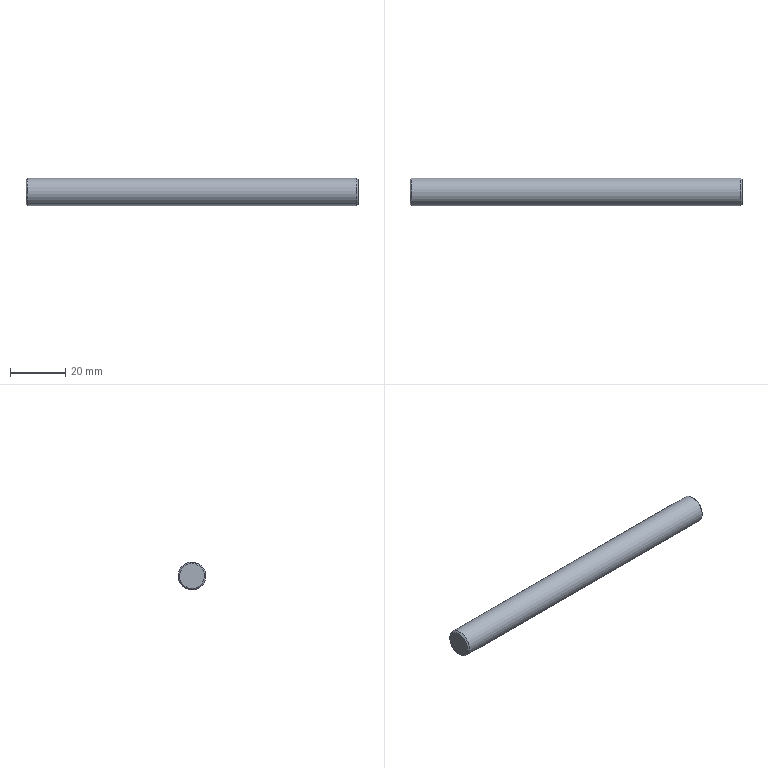Part | STEP file | SN10_016_003_EIXO | 1 solid | 5 faces | box 120 x 10 x 10 mm | volume 9417 mm3 | plane 2 | cone 2 | cylinder 1 | commonest cylinder face diameters 10 x1
STEP:
#1=CARTESIAN_POINT('',(0.,0.,0.));
#2=DIRECTION('',(0.,0.,1.));
#3=DIRECTION('',(1.,0.,0.));
#4=AXIS2_PLACEMENT_3D('',#1,#2,#3);
#5=CARTESIAN_POINT('',(5444.,-1247.157,76.449));
#6=VERTEX_POINT('',#5);
#7=CARTESIAN_POINT('',(5444.,-1245.,72.5));
#8=DIRECTION('',(1.,0.,0.));
#9=DIRECTION('',(0.,1.,0.));
#10=AXIS2_PLACEMENT_3D('',#7,#8,#9);
#11=CIRCLE('',#10,4.5);
#12=CARTESIAN_POINT('',(5444.,-1245.,72.5));
#13=DIRECTION('',(1.,0.,0.));
#14=DIRECTION('',(0.,0.,-1.));
#15=AXIS2_PLACEMENT_3D('',#12,#13,#14);
#16=PLANE('',#15);
#17=CARTESIAN_POINT('',(0.,0.));
#18=DIRECTION('',(0.,1.));
#19=AXIS2_PLACEMENT_2D('',#17,#18);
#20=CIRCLE('',#19,4.5);
#21=(GEOMETRIC_REPRESENTATION_CONTEXT(2)PARAMETRIC_REPRESENTATION_CONTEXT()REPRESENTATION_CONTEXT('',''));
#22=DEFINITIONAL_REPRESENTATION('',(#20),#21);
#23=PCURVE('',#16,#22);
#24=CARTESIAN_POINT('',(5447.5,-1245.,72.5));
#25=DIRECTION('',(-1.,0.,0.));
#26=DIRECTION('',(0.,0.1094,-0.994));
#27=AXIS2_PLACEMENT_3D('',#24,#25,#26);
#28=CONICAL_SURFACE('',#27,1.,0.7854);
#29=CARTESIAN_POINT('',(11.105,3.5));
#30=DIRECTION('',(-1.,0.));
#31=VECTOR('',#30,1.);
#32=LINE('',#29,#31);
#33=(GEOMETRIC_REPRESENTATION_CONTEXT(2)PARAMETRIC_REPRESENTATION_CONTEXT()REPRESENTATION_CONTEXT('',''));
#34=DEFINITIONAL_REPRESENTATION('',(#32),#33);
#35=PCURVE('',#28,#34);
#36=SURFACE_CURVE('',#11,(#23,#35),.PCURVE_S1.);
#37=EDGE_CURVE('',#6,#6,#36,.T.);
#38=ORIENTED_EDGE('',*,*,#37,.T.);
#39=EDGE_LOOP('',(#38));
#40=FACE_BOUND('',#39,.T.);
#41=ADVANCED_FACE('',(#40),#16,.T.);
#42=ORIENTED_EDGE('',*,*,#37,.F.);
#43=CARTESIAN_POINT('',(5443.5,-1247.397,76.888));
#44=VERTEX_POINT('',#43);
#45=CARTESIAN_POINT('',(5444.,-1247.157,76.449));
#46=CARTESIAN_POINT('',(5443.5,-1247.397,76.888));
#47=B_SPLINE_CURVE_WITH_KNOTS('',1,(#45,#46),.UNSPECIFIED.,.F.,.F.,(2,2),(4.95,5.657),.PIECEWISE_BEZIER_KNOTS.);
#48=CARTESIAN_POINT('',(9.034,0.));
#49=DIRECTION('',(0.,1.));
#50=VECTOR('',#49,1.);
#51=LINE('',#48,#50);
#52=(GEOMETRIC_REPRESENTATION_CONTEXT(2)PARAMETRIC_REPRESENTATION_CONTEXT()REPRESENTATION_CONTEXT('',''));
#53=DEFINITIONAL_REPRESENTATION('',(#51),#52);
#54=PCURVE('',#28,#53);
#55=CARTESIAN_POINT('',(2.751,0.));
#56=DIRECTION('',(0.,1.));
#57=VECTOR('',#56,1.);
#58=LINE('',#55,#57);
#59=(GEOMETRIC_REPRESENTATION_CONTEXT(2)PARAMETRIC_REPRESENTATION_CONTEXT()REPRESENTATION_CONTEXT('',''));
#60=DEFINITIONAL_REPRESENTATION('',(#58),#59);
#61=PCURVE('',#28,#60);
#62=SEAM_CURVE('',#47,(#54,#61),.PCURVE_S1.);
#63=EDGE_CURVE('',#6,#44,#62,.T.);
#64=ORIENTED_EDGE('',*,*,#63,.T.);
#65=CARTESIAN_POINT('',(5443.5,-1245.,72.5));
#66=DIRECTION('',(1.,0.,0.));
#67=DIRECTION('',(0.,1.,0.));
#68=AXIS2_PLACEMENT_3D('',#65,#66,#67);
#69=CIRCLE('',#68,5.);
#70=CARTESIAN_POINT('',(11.105,4.));
#71=DIRECTION('',(-1.,0.));
#72=VECTOR('',#71,1.);
#73=LINE('',#70,#72);
#74=(GEOMETRIC_REPRESENTATION_CONTEXT(2)PARAMETRIC_REPRESENTATION_CONTEXT()REPRESENTATION_CONTEXT('',''));
#75=DEFINITIONAL_REPRESENTATION('',(#73),#74);
#76=PCURVE('',#28,#75);
#77=CARTESIAN_POINT('',(5384.,-1245.,72.5));
#78=DIRECTION('',(1.,0.,0.));
#79=DIRECTION('',(0.,-0.4794,0.8776));
#80=AXIS2_PLACEMENT_3D('',#77,#78,#79);
#81=CYLINDRICAL_SURFACE('',#80,5.);
#82=CARTESIAN_POINT('',(-2.071,59.5));
#83=DIRECTION('',(1.,0.));
#84=VECTOR('',#83,1.);
#85=LINE('',#82,#84);
#86=(GEOMETRIC_REPRESENTATION_CONTEXT(2)PARAMETRIC_REPRESENTATION_CONTEXT()REPRESENTATION_CONTEXT('',''));
#87=DEFINITIONAL_REPRESENTATION('',(#85),#86);
#88=PCURVE('',#81,#87);
#89=SURFACE_CURVE('',#69,(#76,#88),.PCURVE_S1.);
#90=EDGE_CURVE('',#44,#44,#89,.T.);
#91=ORIENTED_EDGE('',*,*,#90,.T.);
#92=ORIENTED_EDGE('',*,*,#63,.F.);
#93=EDGE_LOOP('',(#42,#64,#91,#92));
#94=FACE_BOUND('',#93,.T.);
#95=ADVANCED_FACE('',(#94),#28,.T.);
#96=CARTESIAN_POINT('',(5324.,-1247.157,76.449));
#97=VERTEX_POINT('',#96);
#98=CARTESIAN_POINT('',(5324.,-1245.,72.5));
#99=DIRECTION('',(1.,0.,0.));
#100=DIRECTION('',(0.,1.,0.));
#101=AXIS2_PLACEMENT_3D('',#98,#99,#100);
#102=CIRCLE('',#101,4.5);
#103=CARTESIAN_POINT('',(5324.,-1245.,77.5));
#104=DIRECTION('',(1.,0.,0.));
#105=DIRECTION('',(0.,0.,-1.));
#106=AXIS2_PLACEMENT_3D('',#103,#104,#105);
#107=PLANE('',#106);
#108=CARTESIAN_POINT('',(5.,0.));
#109=DIRECTION('',(0.,1.));
#110=AXIS2_PLACEMENT_2D('',#108,#109);
#111=CIRCLE('',#110,4.5);
#112=(GEOMETRIC_REPRESENTATION_CONTEXT(2)PARAMETRIC_REPRESENTATION_CONTEXT()REPRESENTATION_CONTEXT('',''));
#113=DEFINITIONAL_REPRESENTATION('',(#111),#112);
#114=PCURVE('',#107,#113);
#115=CARTESIAN_POINT('',(5320.5,-1245.,72.5));
#116=DIRECTION('',(1.,0.,0.));
#117=DIRECTION('',(0.,-0.128,-0.9918));
#118=AXIS2_PLACEMENT_3D('',#115,#116,#117);
#119=CONICAL_SURFACE('',#118,1.,0.7854);
#120=CARTESIAN_POINT('',(1.699,3.5));
#121=DIRECTION('',(1.,0.));
#122=VECTOR('',#121,1.);
#123=LINE('',#120,#122);
#124=(GEOMETRIC_REPRESENTATION_CONTEXT(2)PARAMETRIC_REPRESENTATION_CONTEXT()REPRESENTATION_CONTEXT('',''));
#125=DEFINITIONAL_REPRESENTATION('',(#123),#124);
#126=PCURVE('',#119,#125);
#127=SURFACE_CURVE('',#102,(#114,#126),.PCURVE_S1.);
#128=EDGE_CURVE('',#97,#97,#127,.T.);
#129=ORIENTED_EDGE('',*,*,#128,.F.);
#130=EDGE_LOOP('',(#129));
#131=FACE_BOUND('',#130,.T.);
#132=ADVANCED_FACE('',(#131),#107,.F.);
#133=CARTESIAN_POINT('',(5324.5,-1247.397,76.888));
#134=VERTEX_POINT('',#133);
#135=CARTESIAN_POINT('',(5324.5,-1245.,72.5));
#136=DIRECTION('',(1.,0.,0.));
#137=DIRECTION('',(0.,1.,0.));
#138=AXIS2_PLACEMENT_3D('',#135,#136,#137);
#139=CIRCLE('',#138,5.);
#140=CARTESIAN_POINT('',(-2.071,-59.5));
#141=DIRECTION('',(1.,0.));
#142=VECTOR('',#141,1.);
#143=LINE('',#140,#142);
#144=(GEOMETRIC_REPRESENTATION_CONTEXT(2)PARAMETRIC_REPRESENTATION_CONTEXT()REPRESENTATION_CONTEXT('',''));
#145=DEFINITIONAL_REPRESENTATION('',(#143),#144);
#146=PCURVE('',#81,#145);
#147=CARTESIAN_POINT('',(1.699,4.));
#148=DIRECTION('',(1.,0.));
#149=VECTOR('',#148,1.);
#150=LINE('',#147,#149);
#151=(GEOMETRIC_REPRESENTATION_CONTEXT(2)PARAMETRIC_REPRESENTATION_CONTEXT()REPRESENTATION_CONTEXT('',''));
#152=DEFINITIONAL_REPRESENTATION('',(#150),#151);
#153=PCURVE('',#119,#152);
#154=SURFACE_CURVE('',#139,(#146,#153),.PCURVE_S1.);
#155=EDGE_CURVE('',#134,#134,#154,.T.);
#156=ORIENTED_EDGE('',*,*,#155,.T.);
#157=CARTESIAN_POINT('',(5324.5,-1247.397,76.888));
#158=CARTESIAN_POINT('',(5443.5,-1247.397,76.888));
#159=B_SPLINE_CURVE_WITH_KNOTS('',1,(#157,#158),.UNSPECIFIED.,.F.,.F.,(2,2),(-59.5,59.5),.PIECEWISE_BEZIER_KNOTS.);
#160=CARTESIAN_POINT('',(6.283,0.));
#161=DIRECTION('',(0.,1.));
#162=VECTOR('',#161,1.);
#163=LINE('',#160,#162);
#164=(GEOMETRIC_REPRESENTATION_CONTEXT(2)PARAMETRIC_REPRESENTATION_CONTEXT()REPRESENTATION_CONTEXT('',''));
#165=DEFINITIONAL_REPRESENTATION('',(#163),#164);
#166=PCURVE('',#81,#165);
#167=CARTESIAN_POINT('',(0.,0.));
#168=DIRECTION('',(0.,1.));
#169=VECTOR('',#168,1.);
#170=LINE('',#167,#169);
#171=(GEOMETRIC_REPRESENTATION_CONTEXT(2)PARAMETRIC_REPRESENTATION_CONTEXT()REPRESENTATION_CONTEXT('',''));
#172=DEFINITIONAL_REPRESENTATION('',(#170),#171);
#173=PCURVE('',#81,#172);
#174=SEAM_CURVE('',#159,(#166,#173),.PCURVE_S1.);
#175=EDGE_CURVE('',#134,#44,#174,.T.);
#176=ORIENTED_EDGE('',*,*,#175,.T.);
#177=ORIENTED_EDGE('',*,*,#90,.F.);
#178=ORIENTED_EDGE('',*,*,#175,.F.);
#179=EDGE_LOOP('',(#156,#176,#177,#178));
#180=FACE_BOUND('',#179,.T.);
#181=ADVANCED_FACE('',(#180),#81,.T.);
#182=ORIENTED_EDGE('',*,*,#155,.F.);
#183=CARTESIAN_POINT('',(5324.,-1247.157,76.449));
#184=CARTESIAN_POINT('',(5324.5,-1247.397,76.888));
#185=B_SPLINE_CURVE_WITH_KNOTS('',1,(#183,#184),.UNSPECIFIED.,.F.,.F.,(2,2),(4.95,5.657),.PIECEWISE_BEZIER_KNOTS.);
#186=CARTESIAN_POINT('',(3.77,0.));
#187=DIRECTION('',(0.,1.));
#188=VECTOR('',#187,1.);
#189=LINE('',#186,#188);
#190=(GEOMETRIC_REPRESENTATION_CONTEXT(2)PARAMETRIC_REPRESENTATION_CONTEXT()REPRESENTATION_CONTEXT('',''));
#191=DEFINITIONAL_REPRESENTATION('',(#189),#190);
#192=PCURVE('',#119,#191);
#193=CARTESIAN_POINT('',(10.053,0.));
#194=DIRECTION('',(0.,1.));
#195=VECTOR('',#194,1.);
#196=LINE('',#193,#195);
#197=(GEOMETRIC_REPRESENTATION_CONTEXT(2)PARAMETRIC_REPRESENTATION_CONTEXT()REPRESENTATION_CONTEXT('',''));
#198=DEFINITIONAL_REPRESENTATION('',(#196),#197);
#199=PCURVE('',#119,#198);
#200=SEAM_CURVE('',#185,(#192,#199),.PCURVE_S1.);
#201=EDGE_CURVE('',#97,#134,#200,.T.);
#202=ORIENTED_EDGE('',*,*,#201,.F.);
#203=ORIENTED_EDGE('',*,*,#128,.T.);
#204=ORIENTED_EDGE('',*,*,#201,.T.);
#205=EDGE_LOOP('',(#182,#202,#203,#204));
#206=FACE_BOUND('',#205,.T.);
#207=ADVANCED_FACE('',(#206),#119,.T.);
#208=CLOSED_SHELL('',(#41,#95,#132,#181,#207));
#209=MANIFOLD_SOLID_BREP('',#208);
#210=(LENGTH_UNIT()NAMED_UNIT(*)SI_UNIT(.MILLI.,.METRE.));
#211=UNCERTAINTY_MEASURE_WITH_UNIT(LENGTH_MEASURE(0.00001),#210,'','');
#212=(NAMED_UNIT(*)PLANE_ANGLE_UNIT()SI_UNIT($,.RADIAN.));
#213=(NAMED_UNIT(*)SI_UNIT($,.STERADIAN.)SOLID_ANGLE_UNIT());
#214=(GEOMETRIC_REPRESENTATION_CONTEXT(3)GLOBAL_UNCERTAINTY_ASSIGNED_CONTEXT((#211))GLOBAL_UNIT_ASSIGNED_CONTEXT((#210,#212,#213))REPRESENTATION_CONTEXT('',''));
#215=ADVANCED_BREP_SHAPE_REPRESENTATION('',(#4,#209),#214);